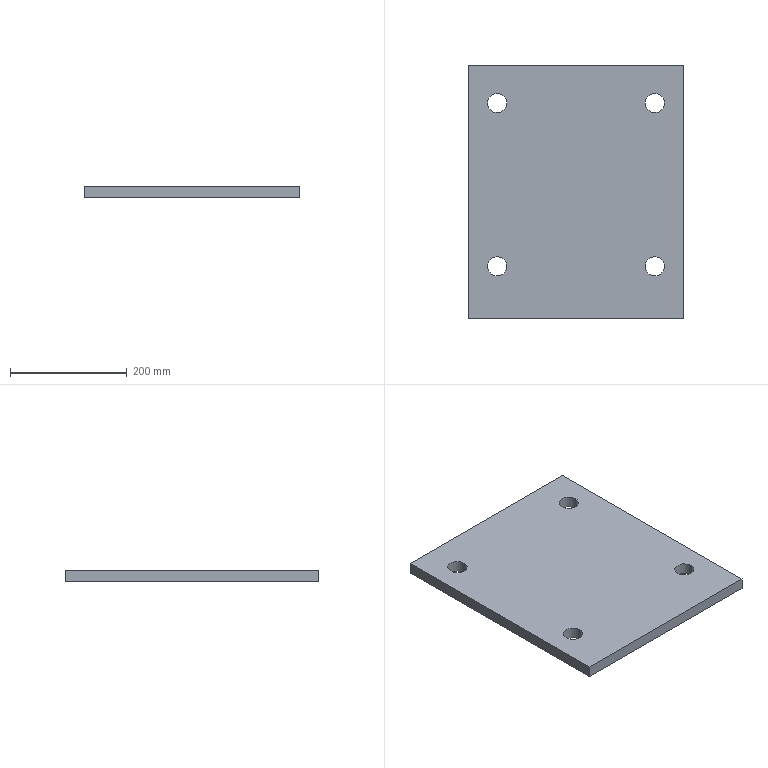Part | STEP file | Motor fixing plate | 1 solid | 14 faces | box 370 x 435 x 20 mm | volume 3150576 mm3 | cylinder 8 | plane 6 | commonest cylinder face diameters 33 x8
STEP:
#1=CARTESIAN_POINT('',(0.,0.,0.));
#2=DIRECTION('',(0.,0.,1.));
#3=DIRECTION('',(1.,0.,0.));
#4=AXIS2_PLACEMENT_3D('',#1,#2,#3);
#5=CARTESIAN_POINT('',(33.5,-345.,20.));
#6=VERTEX_POINT('',#5);
#7=CARTESIAN_POINT('',(33.5,-345.,0.));
#8=VERTEX_POINT('',#7);
#9=CARTESIAN_POINT('',(33.5,-345.,20.));
#10=DIRECTION('',(0.,0.,-1.));
#11=VECTOR('',#10,1.);
#12=LINE('',#9,#11);
#13=CARTESIAN_POINT('',(50.,-345.,20.));
#14=DIRECTION('',(0.,0.,-1.));
#15=DIRECTION('',(-1.,0.,0.));
#16=AXIS2_PLACEMENT_3D('',#13,#14,#15);
#17=CYLINDRICAL_SURFACE('',#16,16.5);
#18=CARTESIAN_POINT('',(6.283,0.));
#19=DIRECTION('',(0.,1.));
#20=VECTOR('',#19,1.);
#21=LINE('',#18,#20);
#22=(GEOMETRIC_REPRESENTATION_CONTEXT(2)PARAMETRIC_REPRESENTATION_CONTEXT()REPRESENTATION_CONTEXT('',''));
#23=DEFINITIONAL_REPRESENTATION('',(#21),#22);
#24=PCURVE('',#17,#23);
#25=CARTESIAN_POINT('',(50.,-345.,20.));
#26=DIRECTION('',(0.,0.,-1.));
#27=DIRECTION('',(-1.,0.,0.));
#28=AXIS2_PLACEMENT_3D('',#25,#26,#27);
#29=CYLINDRICAL_SURFACE('',#28,16.5);
#30=CARTESIAN_POINT('',(0.,0.));
#31=DIRECTION('',(0.,1.));
#32=VECTOR('',#31,1.);
#33=LINE('',#30,#32);
#34=(GEOMETRIC_REPRESENTATION_CONTEXT(2)PARAMETRIC_REPRESENTATION_CONTEXT()REPRESENTATION_CONTEXT('',''));
#35=DEFINITIONAL_REPRESENTATION('',(#33),#34);
#36=PCURVE('',#29,#35);
#37=SURFACE_CURVE('',#12,(#24,#36),.PCURVE_S1.);
#38=EDGE_CURVE('',#6,#8,#37,.T.);
#39=ORIENTED_EDGE('',*,*,#38,.T.);
#40=CARTESIAN_POINT('',(66.5,-345.,0.));
#41=VERTEX_POINT('',#40);
#42=CARTESIAN_POINT('',(50.,-345.,0.));
#43=DIRECTION('',(0.,0.,1.));
#44=DIRECTION('',(1.,0.,0.));
#45=AXIS2_PLACEMENT_3D('',#42,#43,#44);
#46=CIRCLE('',#45,16.5);
#47=CARTESIAN_POINT('',(9.425,20.));
#48=DIRECTION('',(-1.,0.));
#49=VECTOR('',#48,1.);
#50=LINE('',#47,#49);
#51=(GEOMETRIC_REPRESENTATION_CONTEXT(2)PARAMETRIC_REPRESENTATION_CONTEXT()REPRESENTATION_CONTEXT('',''));
#52=DEFINITIONAL_REPRESENTATION('',(#50),#51);
#53=PCURVE('',#17,#52);
#54=CARTESIAN_POINT('',(0.,0.,0.));
#55=DIRECTION('',(0.,0.,1.));
#56=DIRECTION('',(1.,0.,0.));
#57=AXIS2_PLACEMENT_3D('',#54,#55,#56);
#58=PLANE('',#57);
#59=CARTESIAN_POINT('',(50.,-345.));
#60=DIRECTION('',(1.,0.));
#61=AXIS2_PLACEMENT_2D('',#59,#60);
#62=CIRCLE('',#61,16.5);
#63=(GEOMETRIC_REPRESENTATION_CONTEXT(2)PARAMETRIC_REPRESENTATION_CONTEXT()REPRESENTATION_CONTEXT('',''));
#64=DEFINITIONAL_REPRESENTATION('',(#62),#63);
#65=PCURVE('',#58,#64);
#66=SURFACE_CURVE('',#46,(#53,#65),.PCURVE_S1.);
#67=EDGE_CURVE('',#8,#41,#66,.T.);
#68=ORIENTED_EDGE('',*,*,#67,.T.);
#69=CARTESIAN_POINT('',(66.5,-345.,20.));
#70=VERTEX_POINT('',#69);
#71=CARTESIAN_POINT('',(66.5,-345.,20.));
#72=DIRECTION('',(0.,0.,-1.));
#73=VECTOR('',#72,1.);
#74=LINE('',#71,#73);
#75=CARTESIAN_POINT('',(3.142,0.));
#76=DIRECTION('',(0.,1.));
#77=VECTOR('',#76,1.);
#78=LINE('',#75,#77);
#79=(GEOMETRIC_REPRESENTATION_CONTEXT(2)PARAMETRIC_REPRESENTATION_CONTEXT()REPRESENTATION_CONTEXT('',''));
#80=DEFINITIONAL_REPRESENTATION('',(#78),#79);
#81=PCURVE('',#17,#80);
#82=CARTESIAN_POINT('',(3.142,0.));
#83=DIRECTION('',(0.,1.));
#84=VECTOR('',#83,1.);
#85=LINE('',#82,#84);
#86=(GEOMETRIC_REPRESENTATION_CONTEXT(2)PARAMETRIC_REPRESENTATION_CONTEXT()REPRESENTATION_CONTEXT('',''));
#87=DEFINITIONAL_REPRESENTATION('',(#85),#86);
#88=PCURVE('',#29,#87);
#89=SURFACE_CURVE('',#74,(#81,#88),.PCURVE_S1.);
#90=EDGE_CURVE('',#70,#41,#89,.T.);
#91=ORIENTED_EDGE('',*,*,#90,.F.);
#92=CARTESIAN_POINT('',(50.,-345.,20.));
#93=DIRECTION('',(0.,0.,1.));
#94=DIRECTION('',(1.,0.,0.));
#95=AXIS2_PLACEMENT_3D('',#92,#93,#94);
#96=CIRCLE('',#95,16.5);
#97=CARTESIAN_POINT('',(9.425,0.));
#98=DIRECTION('',(-1.,0.));
#99=VECTOR('',#98,1.);
#100=LINE('',#97,#99);
#101=(GEOMETRIC_REPRESENTATION_CONTEXT(2)PARAMETRIC_REPRESENTATION_CONTEXT()REPRESENTATION_CONTEXT('',''));
#102=DEFINITIONAL_REPRESENTATION('',(#100),#101);
#103=PCURVE('',#17,#102);
#104=CARTESIAN_POINT('',(0.,0.,20.));
#105=DIRECTION('',(0.,0.,1.));
#106=DIRECTION('',(1.,0.,0.));
#107=AXIS2_PLACEMENT_3D('',#104,#105,#106);
#108=PLANE('',#107);
#109=CARTESIAN_POINT('',(50.,-345.));
#110=DIRECTION('',(1.,0.));
#111=AXIS2_PLACEMENT_2D('',#109,#110);
#112=CIRCLE('',#111,16.5);
#113=(GEOMETRIC_REPRESENTATION_CONTEXT(2)PARAMETRIC_REPRESENTATION_CONTEXT()REPRESENTATION_CONTEXT('',''));
#114=DEFINITIONAL_REPRESENTATION('',(#112),#113);
#115=PCURVE('',#108,#114);
#116=SURFACE_CURVE('',#96,(#103,#115),.PCURVE_S1.);
#117=EDGE_CURVE('',#6,#70,#116,.T.);
#118=ORIENTED_EDGE('',*,*,#117,.F.);
#119=EDGE_LOOP('',(#39,#68,#91,#118));
#120=FACE_BOUND('',#119,.F.);
#121=ADVANCED_FACE('',(#120),#17,.F.);
#122=CARTESIAN_POINT('',(303.5,-345.,20.));
#123=VERTEX_POINT('',#122);
#124=CARTESIAN_POINT('',(303.5,-345.,0.));
#125=VERTEX_POINT('',#124);
#126=CARTESIAN_POINT('',(303.5,-345.,20.));
#127=DIRECTION('',(0.,0.,-1.));
#128=VECTOR('',#127,1.);
#129=LINE('',#126,#128);
#130=CARTESIAN_POINT('',(320.,-345.,20.));
#131=DIRECTION('',(0.,0.,-1.));
#132=DIRECTION('',(-1.,0.,0.));
#133=AXIS2_PLACEMENT_3D('',#130,#131,#132);
#134=CYLINDRICAL_SURFACE('',#133,16.5);
#135=CARTESIAN_POINT('',(6.283,0.));
#136=DIRECTION('',(0.,1.));
#137=VECTOR('',#136,1.);
#138=LINE('',#135,#137);
#139=(GEOMETRIC_REPRESENTATION_CONTEXT(2)PARAMETRIC_REPRESENTATION_CONTEXT()REPRESENTATION_CONTEXT('',''));
#140=DEFINITIONAL_REPRESENTATION('',(#138),#139);
#141=PCURVE('',#134,#140);
#142=CARTESIAN_POINT('',(320.,-345.,20.));
#143=DIRECTION('',(0.,0.,-1.));
#144=DIRECTION('',(-1.,0.,0.));
#145=AXIS2_PLACEMENT_3D('',#142,#143,#144);
#146=CYLINDRICAL_SURFACE('',#145,16.5);
#147=CARTESIAN_POINT('',(0.,0.));
#148=DIRECTION('',(0.,1.));
#149=VECTOR('',#148,1.);
#150=LINE('',#147,#149);
#151=(GEOMETRIC_REPRESENTATION_CONTEXT(2)PARAMETRIC_REPRESENTATION_CONTEXT()REPRESENTATION_CONTEXT('',''));
#152=DEFINITIONAL_REPRESENTATION('',(#150),#151);
#153=PCURVE('',#146,#152);
#154=SURFACE_CURVE('',#129,(#141,#153),.PCURVE_S1.);
#155=EDGE_CURVE('',#123,#125,#154,.T.);
#156=ORIENTED_EDGE('',*,*,#155,.T.);
#157=CARTESIAN_POINT('',(336.5,-345.,0.));
#158=VERTEX_POINT('',#157);
#159=CARTESIAN_POINT('',(320.,-345.,0.));
#160=DIRECTION('',(0.,0.,1.));
#161=DIRECTION('',(1.,0.,0.));
#162=AXIS2_PLACEMENT_3D('',#159,#160,#161);
#163=CIRCLE('',#162,16.5);
#164=CARTESIAN_POINT('',(9.425,20.));
#165=DIRECTION('',(-1.,0.));
#166=VECTOR('',#165,1.);
#167=LINE('',#164,#166);
#168=(GEOMETRIC_REPRESENTATION_CONTEXT(2)PARAMETRIC_REPRESENTATION_CONTEXT()REPRESENTATION_CONTEXT('',''));
#169=DEFINITIONAL_REPRESENTATION('',(#167),#168);
#170=PCURVE('',#134,#169);
#171=CARTESIAN_POINT('',(320.,-345.));
#172=DIRECTION('',(1.,0.));
#173=AXIS2_PLACEMENT_2D('',#171,#172);
#174=CIRCLE('',#173,16.5);
#175=(GEOMETRIC_REPRESENTATION_CONTEXT(2)PARAMETRIC_REPRESENTATION_CONTEXT()REPRESENTATION_CONTEXT('',''));
#176=DEFINITIONAL_REPRESENTATION('',(#174),#175);
#177=PCURVE('',#58,#176);
#178=SURFACE_CURVE('',#163,(#170,#177),.PCURVE_S1.);
#179=EDGE_CURVE('',#125,#158,#178,.T.);
#180=ORIENTED_EDGE('',*,*,#179,.T.);
#181=CARTESIAN_POINT('',(336.5,-345.,20.));
#182=VERTEX_POINT('',#181);
#183=CARTESIAN_POINT('',(336.5,-345.,20.));
#184=DIRECTION('',(0.,0.,-1.));
#185=VECTOR('',#184,1.);
#186=LINE('',#183,#185);
#187=CARTESIAN_POINT('',(3.142,0.));
#188=DIRECTION('',(0.,1.));
#189=VECTOR('',#188,1.);
#190=LINE('',#187,#189);
#191=(GEOMETRIC_REPRESENTATION_CONTEXT(2)PARAMETRIC_REPRESENTATION_CONTEXT()REPRESENTATION_CONTEXT('',''));
#192=DEFINITIONAL_REPRESENTATION('',(#190),#191);
#193=PCURVE('',#134,#192);
#194=CARTESIAN_POINT('',(3.142,0.));
#195=DIRECTION('',(0.,1.));
#196=VECTOR('',#195,1.);
#197=LINE('',#194,#196);
#198=(GEOMETRIC_REPRESENTATION_CONTEXT(2)PARAMETRIC_REPRESENTATION_CONTEXT()REPRESENTATION_CONTEXT('',''));
#199=DEFINITIONAL_REPRESENTATION('',(#197),#198);
#200=PCURVE('',#146,#199);
#201=SURFACE_CURVE('',#186,(#193,#200),.PCURVE_S1.);
#202=EDGE_CURVE('',#182,#158,#201,.T.);
#203=ORIENTED_EDGE('',*,*,#202,.F.);
#204=CARTESIAN_POINT('',(320.,-345.,20.));
#205=DIRECTION('',(0.,0.,1.));
#206=DIRECTION('',(1.,0.,0.));
#207=AXIS2_PLACEMENT_3D('',#204,#205,#206);
#208=CIRCLE('',#207,16.5);
#209=CARTESIAN_POINT('',(9.425,0.));
#210=DIRECTION('',(-1.,0.));
#211=VECTOR('',#210,1.);
#212=LINE('',#209,#211);
#213=(GEOMETRIC_REPRESENTATION_CONTEXT(2)PARAMETRIC_REPRESENTATION_CONTEXT()REPRESENTATION_CONTEXT('',''));
#214=DEFINITIONAL_REPRESENTATION('',(#212),#213);
#215=PCURVE('',#134,#214);
#216=CARTESIAN_POINT('',(320.,-345.));
#217=DIRECTION('',(1.,0.));
#218=AXIS2_PLACEMENT_2D('',#216,#217);
#219=CIRCLE('',#218,16.5);
#220=(GEOMETRIC_REPRESENTATION_CONTEXT(2)PARAMETRIC_REPRESENTATION_CONTEXT()REPRESENTATION_CONTEXT('',''));
#221=DEFINITIONAL_REPRESENTATION('',(#219),#220);
#222=PCURVE('',#108,#221);
#223=SURFACE_CURVE('',#208,(#215,#222),.PCURVE_S1.);
#224=EDGE_CURVE('',#123,#182,#223,.T.);
#225=ORIENTED_EDGE('',*,*,#224,.F.);
#226=EDGE_LOOP('',(#156,#180,#203,#225));
#227=FACE_BOUND('',#226,.F.);
#228=ADVANCED_FACE('',(#227),#134,.F.);
#229=CARTESIAN_POINT('',(303.5,-65.,20.));
#230=VERTEX_POINT('',#229);
#231=CARTESIAN_POINT('',(303.5,-65.,0.));
#232=VERTEX_POINT('',#231);
#233=CARTESIAN_POINT('',(303.5,-65.,20.));
#234=DIRECTION('',(0.,0.,-1.));
#235=VECTOR('',#234,1.);
#236=LINE('',#233,#235);
#237=CARTESIAN_POINT('',(320.,-65.,20.));
#238=DIRECTION('',(0.,0.,-1.));
#239=DIRECTION('',(-1.,0.,0.));
#240=AXIS2_PLACEMENT_3D('',#237,#238,#239);
#241=CYLINDRICAL_SURFACE('',#240,16.5);
#242=CARTESIAN_POINT('',(6.283,0.));
#243=DIRECTION('',(0.,1.));
#244=VECTOR('',#243,1.);
#245=LINE('',#242,#244);
#246=(GEOMETRIC_REPRESENTATION_CONTEXT(2)PARAMETRIC_REPRESENTATION_CONTEXT()REPRESENTATION_CONTEXT('',''));
#247=DEFINITIONAL_REPRESENTATION('',(#245),#246);
#248=PCURVE('',#241,#247);
#249=CARTESIAN_POINT('',(320.,-65.,20.));
#250=DIRECTION('',(0.,0.,-1.));
#251=DIRECTION('',(-1.,0.,0.));
#252=AXIS2_PLACEMENT_3D('',#249,#250,#251);
#253=CYLINDRICAL_SURFACE('',#252,16.5);
#254=CARTESIAN_POINT('',(0.,0.));
#255=DIRECTION('',(0.,1.));
#256=VECTOR('',#255,1.);
#257=LINE('',#254,#256);
#258=(GEOMETRIC_REPRESENTATION_CONTEXT(2)PARAMETRIC_REPRESENTATION_CONTEXT()REPRESENTATION_CONTEXT('',''));
#259=DEFINITIONAL_REPRESENTATION('',(#257),#258);
#260=PCURVE('',#253,#259);
#261=SURFACE_CURVE('',#236,(#248,#260),.PCURVE_S1.);
#262=EDGE_CURVE('',#230,#232,#261,.T.);
#263=ORIENTED_EDGE('',*,*,#262,.T.);
#264=CARTESIAN_POINT('',(336.5,-65.,0.));
#265=VERTEX_POINT('',#264);
#266=CARTESIAN_POINT('',(320.,-65.,0.));
#267=DIRECTION('',(0.,0.,1.));
#268=DIRECTION('',(1.,0.,0.));
#269=AXIS2_PLACEMENT_3D('',#266,#267,#268);
#270=CIRCLE('',#269,16.5);
#271=CARTESIAN_POINT('',(9.425,20.));
#272=DIRECTION('',(-1.,0.));
#273=VECTOR('',#272,1.);
#274=LINE('',#271,#273);
#275=(GEOMETRIC_REPRESENTATION_CONTEXT(2)PARAMETRIC_REPRESENTATION_CONTEXT()REPRESENTATION_CONTEXT('',''));
#276=DEFINITIONAL_REPRESENTATION('',(#274),#275);
#277=PCURVE('',#241,#276);
#278=CARTESIAN_POINT('',(320.,-65.));
#279=DIRECTION('',(1.,0.));
#280=AXIS2_PLACEMENT_2D('',#278,#279);
#281=CIRCLE('',#280,16.5);
#282=(GEOMETRIC_REPRESENTATION_CONTEXT(2)PARAMETRIC_REPRESENTATION_CONTEXT()REPRESENTATION_CONTEXT('',''));
#283=DEFINITIONAL_REPRESENTATION('',(#281),#282);
#284=PCURVE('',#58,#283);
#285=SURFACE_CURVE('',#270,(#277,#284),.PCURVE_S1.);
#286=EDGE_CURVE('',#232,#265,#285,.T.);
#287=ORIENTED_EDGE('',*,*,#286,.T.);
#288=CARTESIAN_POINT('',(336.5,-65.,20.));
#289=VERTEX_POINT('',#288);
#290=CARTESIAN_POINT('',(336.5,-65.,20.));
#291=DIRECTION('',(0.,0.,-1.));
#292=VECTOR('',#291,1.);
#293=LINE('',#290,#292);
#294=CARTESIAN_POINT('',(3.142,0.));
#295=DIRECTION('',(0.,1.));
#296=VECTOR('',#295,1.);
#297=LINE('',#294,#296);
#298=(GEOMETRIC_REPRESENTATION_CONTEXT(2)PARAMETRIC_REPRESENTATION_CONTEXT()REPRESENTATION_CONTEXT('',''));
#299=DEFINITIONAL_REPRESENTATION('',(#297),#298);
#300=PCURVE('',#241,#299);
#301=CARTESIAN_POINT('',(3.142,0.));
#302=DIRECTION('',(0.,1.));
#303=VECTOR('',#302,1.);
#304=LINE('',#301,#303);
#305=(GEOMETRIC_REPRESENTATION_CONTEXT(2)PARAMETRIC_REPRESENTATION_CONTEXT()REPRESENTATION_CONTEXT('',''));
#306=DEFINITIONAL_REPRESENTATION('',(#304),#305);
#307=PCURVE('',#253,#306);
#308=SURFACE_CURVE('',#293,(#300,#307),.PCURVE_S1.);
#309=EDGE_CURVE('',#289,#265,#308,.T.);
#310=ORIENTED_EDGE('',*,*,#309,.F.);
#311=CARTESIAN_POINT('',(320.,-65.,20.));
#312=DIRECTION('',(0.,0.,1.));
#313=DIRECTION('',(1.,0.,0.));
#314=AXIS2_PLACEMENT_3D('',#311,#312,#313);
#315=CIRCLE('',#314,16.5);
#316=CARTESIAN_POINT('',(9.425,0.));
#317=DIRECTION('',(-1.,0.));
#318=VECTOR('',#317,1.);
#319=LINE('',#316,#318);
#320=(GEOMETRIC_REPRESENTATION_CONTEXT(2)PARAMETRIC_REPRESENTATION_CONTEXT()REPRESENTATION_CONTEXT('',''));
#321=DEFINITIONAL_REPRESENTATION('',(#319),#320);
#322=PCURVE('',#241,#321);
#323=CARTESIAN_POINT('',(320.,-65.));
#324=DIRECTION('',(1.,0.));
#325=AXIS2_PLACEMENT_2D('',#323,#324);
#326=CIRCLE('',#325,16.5);
#327=(GEOMETRIC_REPRESENTATION_CONTEXT(2)PARAMETRIC_REPRESENTATION_CONTEXT()REPRESENTATION_CONTEXT('',''));
#328=DEFINITIONAL_REPRESENTATION('',(#326),#327);
#329=PCURVE('',#108,#328);
#330=SURFACE_CURVE('',#315,(#322,#329),.PCURVE_S1.);
#331=EDGE_CURVE('',#230,#289,#330,.T.);
#332=ORIENTED_EDGE('',*,*,#331,.F.);
#333=EDGE_LOOP('',(#263,#287,#310,#332));
#334=FACE_BOUND('',#333,.F.);
#335=ADVANCED_FACE('',(#334),#241,.F.);
#336=CARTESIAN_POINT('',(33.5,-65.,20.));
#337=VERTEX_POINT('',#336);
#338=CARTESIAN_POINT('',(33.5,-65.,0.));
#339=VERTEX_POINT('',#338);
#340=CARTESIAN_POINT('',(33.5,-65.,20.));
#341=DIRECTION('',(0.,0.,-1.));
#342=VECTOR('',#341,1.);
#343=LINE('',#340,#342);
#344=CARTESIAN_POINT('',(50.,-65.,20.));
#345=DIRECTION('',(0.,0.,-1.));
#346=DIRECTION('',(-1.,0.,0.));
#347=AXIS2_PLACEMENT_3D('',#344,#345,#346);
#348=CYLINDRICAL_SURFACE('',#347,16.5);
#349=CARTESIAN_POINT('',(6.283,0.));
#350=DIRECTION('',(0.,1.));
#351=VECTOR('',#350,1.);
#352=LINE('',#349,#351);
#353=(GEOMETRIC_REPRESENTATION_CONTEXT(2)PARAMETRIC_REPRESENTATION_CONTEXT()REPRESENTATION_CONTEXT('',''));
#354=DEFINITIONAL_REPRESENTATION('',(#352),#353);
#355=PCURVE('',#348,#354);
#356=CARTESIAN_POINT('',(50.,-65.,20.));
#357=DIRECTION('',(0.,0.,-1.));
#358=DIRECTION('',(-1.,0.,0.));
#359=AXIS2_PLACEMENT_3D('',#356,#357,#358);
#360=CYLINDRICAL_SURFACE('',#359,16.5);
#361=CARTESIAN_POINT('',(0.,0.));
#362=DIRECTION('',(0.,1.));
#363=VECTOR('',#362,1.);
#364=LINE('',#361,#363);
#365=(GEOMETRIC_REPRESENTATION_CONTEXT(2)PARAMETRIC_REPRESENTATION_CONTEXT()REPRESENTATION_CONTEXT('',''));
#366=DEFINITIONAL_REPRESENTATION('',(#364),#365);
#367=PCURVE('',#360,#366);
#368=SURFACE_CURVE('',#343,(#355,#367),.PCURVE_S1.);
#369=EDGE_CURVE('',#337,#339,#368,.T.);
#370=ORIENTED_EDGE('',*,*,#369,.T.);
#371=CARTESIAN_POINT('',(66.5,-65.,0.));
#372=VERTEX_POINT('',#371);
#373=CARTESIAN_POINT('',(50.,-65.,0.));
#374=DIRECTION('',(0.,0.,1.));
#375=DIRECTION('',(1.,0.,0.));
#376=AXIS2_PLACEMENT_3D('',#373,#374,#375);
#377=CIRCLE('',#376,16.5);
#378=CARTESIAN_POINT('',(9.425,20.));
#379=DIRECTION('',(-1.,0.));
#380=VECTOR('',#379,1.);
#381=LINE('',#378,#380);
#382=(GEOMETRIC_REPRESENTATION_CONTEXT(2)PARAMETRIC_REPRESENTATION_CONTEXT()REPRESENTATION_CONTEXT('',''));
#383=DEFINITIONAL_REPRESENTATION('',(#381),#382);
#384=PCURVE('',#348,#383);
#385=CARTESIAN_POINT('',(50.,-65.));
#386=DIRECTION('',(1.,0.));
#387=AXIS2_PLACEMENT_2D('',#385,#386);
#388=CIRCLE('',#387,16.5);
#389=(GEOMETRIC_REPRESENTATION_CONTEXT(2)PARAMETRIC_REPRESENTATION_CONTEXT()REPRESENTATION_CONTEXT('',''));
#390=DEFINITIONAL_REPRESENTATION('',(#388),#389);
#391=PCURVE('',#58,#390);
#392=SURFACE_CURVE('',#377,(#384,#391),.PCURVE_S1.);
#393=EDGE_CURVE('',#339,#372,#392,.T.);
#394=ORIENTED_EDGE('',*,*,#393,.T.);
#395=CARTESIAN_POINT('',(66.5,-65.,20.));
#396=VERTEX_POINT('',#395);
#397=CARTESIAN_POINT('',(66.5,-65.,20.));
#398=DIRECTION('',(0.,0.,-1.));
#399=VECTOR('',#398,1.);
#400=LINE('',#397,#399);
#401=CARTESIAN_POINT('',(3.142,0.));
#402=DIRECTION('',(0.,1.));
#403=VECTOR('',#402,1.);
#404=LINE('',#401,#403);
#405=(GEOMETRIC_REPRESENTATION_CONTEXT(2)PARAMETRIC_REPRESENTATION_CONTEXT()REPRESENTATION_CONTEXT('',''));
#406=DEFINITIONAL_REPRESENTATION('',(#404),#405);
#407=PCURVE('',#348,#406);
#408=CARTESIAN_POINT('',(3.142,0.));
#409=DIRECTION('',(0.,1.));
#410=VECTOR('',#409,1.);
#411=LINE('',#408,#410);
#412=(GEOMETRIC_REPRESENTATION_CONTEXT(2)PARAMETRIC_REPRESENTATION_CONTEXT()REPRESENTATION_CONTEXT('',''));
#413=DEFINITIONAL_REPRESENTATION('',(#411),#412);
#414=PCURVE('',#360,#413);
#415=SURFACE_CURVE('',#400,(#407,#414),.PCURVE_S1.);
#416=EDGE_CURVE('',#396,#372,#415,.T.);
#417=ORIENTED_EDGE('',*,*,#416,.F.);
#418=CARTESIAN_POINT('',(50.,-65.,20.));
#419=DIRECTION('',(0.,0.,1.));
#420=DIRECTION('',(1.,0.,0.));
#421=AXIS2_PLACEMENT_3D('',#418,#419,#420);
#422=CIRCLE('',#421,16.5);
#423=CARTESIAN_POINT('',(9.425,0.));
#424=DIRECTION('',(-1.,0.));
#425=VECTOR('',#424,1.);
#426=LINE('',#423,#425);
#427=(GEOMETRIC_REPRESENTATION_CONTEXT(2)PARAMETRIC_REPRESENTATION_CONTEXT()REPRESENTATION_CONTEXT('',''));
#428=DEFINITIONAL_REPRESENTATION('',(#426),#427);
#429=PCURVE('',#348,#428);
#430=CARTESIAN_POINT('',(50.,-65.));
#431=DIRECTION('',(1.,0.));
#432=AXIS2_PLACEMENT_2D('',#430,#431);
#433=CIRCLE('',#432,16.5);
#434=(GEOMETRIC_REPRESENTATION_CONTEXT(2)PARAMETRIC_REPRESENTATION_CONTEXT()REPRESENTATION_CONTEXT('',''));
#435=DEFINITIONAL_REPRESENTATION('',(#433),#434);
#436=PCURVE('',#108,#435);
#437=SURFACE_CURVE('',#422,(#429,#436),.PCURVE_S1.);
#438=EDGE_CURVE('',#337,#396,#437,.T.);
#439=ORIENTED_EDGE('',*,*,#438,.F.);
#440=EDGE_LOOP('',(#370,#394,#417,#439));
#441=FACE_BOUND('',#440,.F.);
#442=ADVANCED_FACE('',(#441),#348,.F.);
#443=ORIENTED_EDGE('',*,*,#224,.F.);
#444=CARTESIAN_POINT('',(320.,-345.,20.));
#445=DIRECTION('',(0.,0.,1.));
#446=DIRECTION('',(1.,0.,0.));
#447=AXIS2_PLACEMENT_3D('',#444,#445,#446);
#448=CIRCLE('',#447,16.5);
#449=CARTESIAN_POINT('',(320.,-345.));
#450=DIRECTION('',(1.,0.));
#451=AXIS2_PLACEMENT_2D('',#449,#450);
#452=CIRCLE('',#451,16.5);
#453=(GEOMETRIC_REPRESENTATION_CONTEXT(2)PARAMETRIC_REPRESENTATION_CONTEXT()REPRESENTATION_CONTEXT('',''));
#454=DEFINITIONAL_REPRESENTATION('',(#452),#453);
#455=PCURVE('',#108,#454);
#456=CARTESIAN_POINT('',(3.142,0.));
#457=DIRECTION('',(-1.,0.));
#458=VECTOR('',#457,1.);
#459=LINE('',#456,#458);
#460=(GEOMETRIC_REPRESENTATION_CONTEXT(2)PARAMETRIC_REPRESENTATION_CONTEXT()REPRESENTATION_CONTEXT('',''));
#461=DEFINITIONAL_REPRESENTATION('',(#459),#460);
#462=PCURVE('',#146,#461);
#463=SURFACE_CURVE('',#448,(#455,#462),.PCURVE_S1.);
#464=EDGE_CURVE('',#182,#123,#463,.T.);
#465=ORIENTED_EDGE('',*,*,#464,.F.);
#466=EDGE_LOOP('',(#443,#465));
#467=FACE_BOUND('',#466,.T.);
#468=ORIENTED_EDGE('',*,*,#438,.F.);
#469=CARTESIAN_POINT('',(50.,-65.,20.));
#470=DIRECTION('',(0.,0.,1.));
#471=DIRECTION('',(1.,0.,0.));
#472=AXIS2_PLACEMENT_3D('',#469,#470,#471);
#473=CIRCLE('',#472,16.5);
#474=CARTESIAN_POINT('',(50.,-65.));
#475=DIRECTION('',(1.,0.));
#476=AXIS2_PLACEMENT_2D('',#474,#475);
#477=CIRCLE('',#476,16.5);
#478=(GEOMETRIC_REPRESENTATION_CONTEXT(2)PARAMETRIC_REPRESENTATION_CONTEXT()REPRESENTATION_CONTEXT('',''));
#479=DEFINITIONAL_REPRESENTATION('',(#477),#478);
#480=PCURVE('',#108,#479);
#481=CARTESIAN_POINT('',(3.142,0.));
#482=DIRECTION('',(-1.,0.));
#483=VECTOR('',#482,1.);
#484=LINE('',#481,#483);
#485=(GEOMETRIC_REPRESENTATION_CONTEXT(2)PARAMETRIC_REPRESENTATION_CONTEXT()REPRESENTATION_CONTEXT('',''));
#486=DEFINITIONAL_REPRESENTATION('',(#484),#485);
#487=PCURVE('',#360,#486);
#488=SURFACE_CURVE('',#473,(#480,#487),.PCURVE_S1.);
#489=EDGE_CURVE('',#396,#337,#488,.T.);
#490=ORIENTED_EDGE('',*,*,#489,.F.);
#491=EDGE_LOOP('',(#468,#490));
#492=FACE_BOUND('',#491,.T.);
#493=CARTESIAN_POINT('',(0.,0.,20.));
#494=VERTEX_POINT('',#493);
#495=CARTESIAN_POINT('',(0.,-435.,20.));
#496=VERTEX_POINT('',#495);
#497=CARTESIAN_POINT('',(0.,0.,20.));
#498=DIRECTION('',(0.,-1.,0.));
#499=VECTOR('',#498,1.);
#500=LINE('',#497,#499);
#501=CARTESIAN_POINT('',(0.,0.));
#502=DIRECTION('',(0.,-1.));
#503=VECTOR('',#502,1.);
#504=LINE('',#501,#503);
#505=(GEOMETRIC_REPRESENTATION_CONTEXT(2)PARAMETRIC_REPRESENTATION_CONTEXT()REPRESENTATION_CONTEXT('',''));
#506=DEFINITIONAL_REPRESENTATION('',(#504),#505);
#507=PCURVE('',#108,#506);
#508=CARTESIAN_POINT('',(0.,0.,20.));
#509=DIRECTION('',(1.,0.,0.));
#510=DIRECTION('',(0.,1.,0.));
#511=AXIS2_PLACEMENT_3D('',#508,#509,#510);
#512=PLANE('',#511);
#513=CARTESIAN_POINT('',(0.,0.));
#514=DIRECTION('',(-1.,0.));
#515=VECTOR('',#514,1.);
#516=LINE('',#513,#515);
#517=(GEOMETRIC_REPRESENTATION_CONTEXT(2)PARAMETRIC_REPRESENTATION_CONTEXT()REPRESENTATION_CONTEXT('',''));
#518=DEFINITIONAL_REPRESENTATION('',(#516),#517);
#519=PCURVE('',#512,#518);
#520=SURFACE_CURVE('',#500,(#507,#519),.PCURVE_S1.);
#521=EDGE_CURVE('',#494,#496,#520,.T.);
#522=ORIENTED_EDGE('',*,*,#521,.T.);
#523=CARTESIAN_POINT('',(370.,-435.,20.));
#524=VERTEX_POINT('',#523);
#525=CARTESIAN_POINT('',(0.,-435.,20.));
#526=DIRECTION('',(1.,0.,0.));
#527=VECTOR('',#526,1.);
#528=LINE('',#525,#527);
#529=CARTESIAN_POINT('',(0.,-435.));
#530=DIRECTION('',(1.,0.));
#531=VECTOR('',#530,1.);
#532=LINE('',#529,#531);
#533=(GEOMETRIC_REPRESENTATION_CONTEXT(2)PARAMETRIC_REPRESENTATION_CONTEXT()REPRESENTATION_CONTEXT('',''));
#534=DEFINITIONAL_REPRESENTATION('',(#532),#533);
#535=PCURVE('',#108,#534);
#536=CARTESIAN_POINT('',(0.,-435.,20.));
#537=DIRECTION('',(0.,1.,0.));
#538=DIRECTION('',(0.,0.,1.));
#539=AXIS2_PLACEMENT_3D('',#536,#537,#538);
#540=PLANE('',#539);
#541=CARTESIAN_POINT('',(0.,0.));
#542=DIRECTION('',(0.,1.));
#543=VECTOR('',#542,1.);
#544=LINE('',#541,#543);
#545=(GEOMETRIC_REPRESENTATION_CONTEXT(2)PARAMETRIC_REPRESENTATION_CONTEXT()REPRESENTATION_CONTEXT('',''));
#546=DEFINITIONAL_REPRESENTATION('',(#544),#545);
#547=PCURVE('',#540,#546);
#548=SURFACE_CURVE('',#528,(#535,#547),.PCURVE_S1.);
#549=EDGE_CURVE('',#496,#524,#548,.T.);
#550=ORIENTED_EDGE('',*,*,#549,.T.);
#551=CARTESIAN_POINT('',(370.,0.,20.));
#552=VERTEX_POINT('',#551);
#553=CARTESIAN_POINT('',(370.,0.,20.));
#554=DIRECTION('',(0.,1.,0.));
#555=VECTOR('',#554,1.);
#556=LINE('',#553,#555);
#557=CARTESIAN_POINT('',(370.,0.));
#558=DIRECTION('',(0.,1.));
#559=VECTOR('',#558,1.);
#560=LINE('',#557,#559);
#561=(GEOMETRIC_REPRESENTATION_CONTEXT(2)PARAMETRIC_REPRESENTATION_CONTEXT()REPRESENTATION_CONTEXT('',''));
#562=DEFINITIONAL_REPRESENTATION('',(#560),#561);
#563=PCURVE('',#108,#562);
#564=CARTESIAN_POINT('',(370.,0.,20.));
#565=DIRECTION('',(-1.,0.,0.));
#566=DIRECTION('',(0.,-1.,0.));
#567=AXIS2_PLACEMENT_3D('',#564,#565,#566);
#568=PLANE('',#567);
#569=CARTESIAN_POINT('',(0.,0.));
#570=DIRECTION('',(-1.,0.));
#571=VECTOR('',#570,1.);
#572=LINE('',#569,#571);
#573=(GEOMETRIC_REPRESENTATION_CONTEXT(2)PARAMETRIC_REPRESENTATION_CONTEXT()REPRESENTATION_CONTEXT('',''));
#574=DEFINITIONAL_REPRESENTATION('',(#572),#573);
#575=PCURVE('',#568,#574);
#576=SURFACE_CURVE('',#556,(#563,#575),.PCURVE_S1.);
#577=EDGE_CURVE('',#524,#552,#576,.T.);
#578=ORIENTED_EDGE('',*,*,#577,.T.);
#579=CARTESIAN_POINT('',(0.,0.,20.));
#580=DIRECTION('',(-1.,0.,0.));
#581=VECTOR('',#580,1.);
#582=LINE('',#579,#581);
#583=CARTESIAN_POINT('',(0.,0.));
#584=DIRECTION('',(-1.,0.));
#585=VECTOR('',#584,1.);
#586=LINE('',#583,#585);
#587=(GEOMETRIC_REPRESENTATION_CONTEXT(2)PARAMETRIC_REPRESENTATION_CONTEXT()REPRESENTATION_CONTEXT('',''));
#588=DEFINITIONAL_REPRESENTATION('',(#586),#587);
#589=PCURVE('',#108,#588);
#590=CARTESIAN_POINT('',(0.,0.,20.));
#591=DIRECTION('',(0.,-1.,0.));
#592=DIRECTION('',(0.,0.,-1.));
#593=AXIS2_PLACEMENT_3D('',#590,#591,#592);
#594=PLANE('',#593);
#595=CARTESIAN_POINT('',(0.,0.));
#596=DIRECTION('',(0.,-1.));
#597=VECTOR('',#596,1.);
#598=LINE('',#595,#597);
#599=(GEOMETRIC_REPRESENTATION_CONTEXT(2)PARAMETRIC_REPRESENTATION_CONTEXT()REPRESENTATION_CONTEXT('',''));
#600=DEFINITIONAL_REPRESENTATION('',(#598),#599);
#601=PCURVE('',#594,#600);
#602=SURFACE_CURVE('',#582,(#589,#601),.PCURVE_S1.);
#603=EDGE_CURVE('',#552,#494,#602,.T.);
#604=ORIENTED_EDGE('',*,*,#603,.T.);
#605=EDGE_LOOP('',(#522,#550,#578,#604));
#606=FACE_BOUND('',#605,.T.);
#607=ORIENTED_EDGE('',*,*,#331,.F.);
#608=CARTESIAN_POINT('',(320.,-65.,20.));
#609=DIRECTION('',(0.,0.,1.));
#610=DIRECTION('',(1.,0.,0.));
#611=AXIS2_PLACEMENT_3D('',#608,#609,#610);
#612=CIRCLE('',#611,16.5);
#613=CARTESIAN_POINT('',(320.,-65.));
#614=DIRECTION('',(1.,0.));
#615=AXIS2_PLACEMENT_2D('',#613,#614);
#616=CIRCLE('',#615,16.5);
#617=(GEOMETRIC_REPRESENTATION_CONTEXT(2)PARAMETRIC_REPRESENTATION_CONTEXT()REPRESENTATION_CONTEXT('',''));
#618=DEFINITIONAL_REPRESENTATION('',(#616),#617);
#619=PCURVE('',#108,#618);
#620=CARTESIAN_POINT('',(3.142,0.));
#621=DIRECTION('',(-1.,0.));
#622=VECTOR('',#621,1.);
#623=LINE('',#620,#622);
#624=(GEOMETRIC_REPRESENTATION_CONTEXT(2)PARAMETRIC_REPRESENTATION_CONTEXT()REPRESENTATION_CONTEXT('',''));
#625=DEFINITIONAL_REPRESENTATION('',(#623),#624);
#626=PCURVE('',#253,#625);
#627=SURFACE_CURVE('',#612,(#619,#626),.PCURVE_S1.);
#628=EDGE_CURVE('',#289,#230,#627,.T.);
#629=ORIENTED_EDGE('',*,*,#628,.F.);
#630=EDGE_LOOP('',(#607,#629));
#631=FACE_BOUND('',#630,.T.);
#632=ORIENTED_EDGE('',*,*,#117,.F.);
#633=CARTESIAN_POINT('',(50.,-345.,20.));
#634=DIRECTION('',(0.,0.,1.));
#635=DIRECTION('',(1.,0.,0.));
#636=AXIS2_PLACEMENT_3D('',#633,#634,#635);
#637=CIRCLE('',#636,16.5);
#638=CARTESIAN_POINT('',(50.,-345.));
#639=DIRECTION('',(1.,0.));
#640=AXIS2_PLACEMENT_2D('',#638,#639);
#641=CIRCLE('',#640,16.5);
#642=(GEOMETRIC_REPRESENTATION_CONTEXT(2)PARAMETRIC_REPRESENTATION_CONTEXT()REPRESENTATION_CONTEXT('',''));
#643=DEFINITIONAL_REPRESENTATION('',(#641),#642);
#644=PCURVE('',#108,#643);
#645=CARTESIAN_POINT('',(3.142,0.));
#646=DIRECTION('',(-1.,0.));
#647=VECTOR('',#646,1.);
#648=LINE('',#645,#647);
#649=(GEOMETRIC_REPRESENTATION_CONTEXT(2)PARAMETRIC_REPRESENTATION_CONTEXT()REPRESENTATION_CONTEXT('',''));
#650=DEFINITIONAL_REPRESENTATION('',(#648),#649);
#651=PCURVE('',#29,#650);
#652=SURFACE_CURVE('',#637,(#644,#651),.PCURVE_S1.);
#653=EDGE_CURVE('',#70,#6,#652,.T.);
#654=ORIENTED_EDGE('',*,*,#653,.F.);
#655=EDGE_LOOP('',(#632,#654));
#656=FACE_BOUND('',#655,.T.);
#657=ADVANCED_FACE('',(#467,#492,#606,#631,#656),#108,.T.);
#658=ORIENTED_EDGE('',*,*,#179,.T.);
#659=CARTESIAN_POINT('',(320.,-345.,0.));
#660=DIRECTION('',(0.,0.,1.));
#661=DIRECTION('',(1.,0.,0.));
#662=AXIS2_PLACEMENT_3D('',#659,#660,#661);
#663=CIRCLE('',#662,16.5);
#664=CARTESIAN_POINT('',(320.,-345.));
#665=DIRECTION('',(1.,0.));
#666=AXIS2_PLACEMENT_2D('',#664,#665);
#667=CIRCLE('',#666,16.5);
#668=(GEOMETRIC_REPRESENTATION_CONTEXT(2)PARAMETRIC_REPRESENTATION_CONTEXT()REPRESENTATION_CONTEXT('',''));
#669=DEFINITIONAL_REPRESENTATION('',(#667),#668);
#670=PCURVE('',#58,#669);
#671=CARTESIAN_POINT('',(3.142,20.));
#672=DIRECTION('',(-1.,0.));
#673=VECTOR('',#672,1.);
#674=LINE('',#671,#673);
#675=(GEOMETRIC_REPRESENTATION_CONTEXT(2)PARAMETRIC_REPRESENTATION_CONTEXT()REPRESENTATION_CONTEXT('',''));
#676=DEFINITIONAL_REPRESENTATION('',(#674),#675);
#677=PCURVE('',#146,#676);
#678=SURFACE_CURVE('',#663,(#670,#677),.PCURVE_S1.);
#679=EDGE_CURVE('',#158,#125,#678,.T.);
#680=ORIENTED_EDGE('',*,*,#679,.T.);
#681=EDGE_LOOP('',(#658,#680));
#682=FACE_BOUND('',#681,.T.);
#683=ORIENTED_EDGE('',*,*,#393,.T.);
#684=CARTESIAN_POINT('',(50.,-65.,0.));
#685=DIRECTION('',(0.,0.,1.));
#686=DIRECTION('',(1.,0.,0.));
#687=AXIS2_PLACEMENT_3D('',#684,#685,#686);
#688=CIRCLE('',#687,16.5);
#689=CARTESIAN_POINT('',(50.,-65.));
#690=DIRECTION('',(1.,0.));
#691=AXIS2_PLACEMENT_2D('',#689,#690);
#692=CIRCLE('',#691,16.5);
#693=(GEOMETRIC_REPRESENTATION_CONTEXT(2)PARAMETRIC_REPRESENTATION_CONTEXT()REPRESENTATION_CONTEXT('',''));
#694=DEFINITIONAL_REPRESENTATION('',(#692),#693);
#695=PCURVE('',#58,#694);
#696=CARTESIAN_POINT('',(3.142,20.));
#697=DIRECTION('',(-1.,0.));
#698=VECTOR('',#697,1.);
#699=LINE('',#696,#698);
#700=(GEOMETRIC_REPRESENTATION_CONTEXT(2)PARAMETRIC_REPRESENTATION_CONTEXT()REPRESENTATION_CONTEXT('',''));
#701=DEFINITIONAL_REPRESENTATION('',(#699),#700);
#702=PCURVE('',#360,#701);
#703=SURFACE_CURVE('',#688,(#695,#702),.PCURVE_S1.);
#704=EDGE_CURVE('',#372,#339,#703,.T.);
#705=ORIENTED_EDGE('',*,*,#704,.T.);
#706=EDGE_LOOP('',(#683,#705));
#707=FACE_BOUND('',#706,.T.);
#708=CARTESIAN_POINT('',(0.,0.,0.));
#709=VERTEX_POINT('',#708);
#710=CARTESIAN_POINT('',(0.,-435.,0.));
#711=VERTEX_POINT('',#710);
#712=CARTESIAN_POINT('',(0.,0.,0.));
#713=DIRECTION('',(0.,-1.,0.));
#714=VECTOR('',#713,1.);
#715=LINE('',#712,#714);
#716=CARTESIAN_POINT('',(0.,0.));
#717=DIRECTION('',(0.,-1.));
#718=VECTOR('',#717,1.);
#719=LINE('',#716,#718);
#720=(GEOMETRIC_REPRESENTATION_CONTEXT(2)PARAMETRIC_REPRESENTATION_CONTEXT()REPRESENTATION_CONTEXT('',''));
#721=DEFINITIONAL_REPRESENTATION('',(#719),#720);
#722=PCURVE('',#58,#721);
#723=CARTESIAN_POINT('',(0.,-20.));
#724=DIRECTION('',(-1.,0.));
#725=VECTOR('',#724,1.);
#726=LINE('',#723,#725);
#727=(GEOMETRIC_REPRESENTATION_CONTEXT(2)PARAMETRIC_REPRESENTATION_CONTEXT()REPRESENTATION_CONTEXT('',''));
#728=DEFINITIONAL_REPRESENTATION('',(#726),#727);
#729=PCURVE('',#512,#728);
#730=SURFACE_CURVE('',#715,(#722,#729),.PCURVE_S1.);
#731=EDGE_CURVE('',#709,#711,#730,.T.);
#732=ORIENTED_EDGE('',*,*,#731,.F.);
#733=CARTESIAN_POINT('',(370.,0.,0.));
#734=VERTEX_POINT('',#733);
#735=CARTESIAN_POINT('',(0.,0.,0.));
#736=DIRECTION('',(-1.,0.,0.));
#737=VECTOR('',#736,1.);
#738=LINE('',#735,#737);
#739=CARTESIAN_POINT('',(0.,0.));
#740=DIRECTION('',(-1.,0.));
#741=VECTOR('',#740,1.);
#742=LINE('',#739,#741);
#743=(GEOMETRIC_REPRESENTATION_CONTEXT(2)PARAMETRIC_REPRESENTATION_CONTEXT()REPRESENTATION_CONTEXT('',''));
#744=DEFINITIONAL_REPRESENTATION('',(#742),#743);
#745=PCURVE('',#58,#744);
#746=CARTESIAN_POINT('',(20.,0.));
#747=DIRECTION('',(0.,-1.));
#748=VECTOR('',#747,1.);
#749=LINE('',#746,#748);
#750=(GEOMETRIC_REPRESENTATION_CONTEXT(2)PARAMETRIC_REPRESENTATION_CONTEXT()REPRESENTATION_CONTEXT('',''));
#751=DEFINITIONAL_REPRESENTATION('',(#749),#750);
#752=PCURVE('',#594,#751);
#753=SURFACE_CURVE('',#738,(#745,#752),.PCURVE_S1.);
#754=EDGE_CURVE('',#734,#709,#753,.T.);
#755=ORIENTED_EDGE('',*,*,#754,.F.);
#756=CARTESIAN_POINT('',(370.,-435.,0.));
#757=VERTEX_POINT('',#756);
#758=CARTESIAN_POINT('',(370.,0.,0.));
#759=DIRECTION('',(0.,1.,0.));
#760=VECTOR('',#759,1.);
#761=LINE('',#758,#760);
#762=CARTESIAN_POINT('',(370.,0.));
#763=DIRECTION('',(0.,1.));
#764=VECTOR('',#763,1.);
#765=LINE('',#762,#764);
#766=(GEOMETRIC_REPRESENTATION_CONTEXT(2)PARAMETRIC_REPRESENTATION_CONTEXT()REPRESENTATION_CONTEXT('',''));
#767=DEFINITIONAL_REPRESENTATION('',(#765),#766);
#768=PCURVE('',#58,#767);
#769=CARTESIAN_POINT('',(0.,-20.));
#770=DIRECTION('',(-1.,0.));
#771=VECTOR('',#770,1.);
#772=LINE('',#769,#771);
#773=(GEOMETRIC_REPRESENTATION_CONTEXT(2)PARAMETRIC_REPRESENTATION_CONTEXT()REPRESENTATION_CONTEXT('',''));
#774=DEFINITIONAL_REPRESENTATION('',(#772),#773);
#775=PCURVE('',#568,#774);
#776=SURFACE_CURVE('',#761,(#768,#775),.PCURVE_S1.);
#777=EDGE_CURVE('',#757,#734,#776,.T.);
#778=ORIENTED_EDGE('',*,*,#777,.F.);
#779=CARTESIAN_POINT('',(0.,-435.,0.));
#780=DIRECTION('',(1.,0.,0.));
#781=VECTOR('',#780,1.);
#782=LINE('',#779,#781);
#783=CARTESIAN_POINT('',(0.,-435.));
#784=DIRECTION('',(1.,0.));
#785=VECTOR('',#784,1.);
#786=LINE('',#783,#785);
#787=(GEOMETRIC_REPRESENTATION_CONTEXT(2)PARAMETRIC_REPRESENTATION_CONTEXT()REPRESENTATION_CONTEXT('',''));
#788=DEFINITIONAL_REPRESENTATION('',(#786),#787);
#789=PCURVE('',#58,#788);
#790=CARTESIAN_POINT('',(-20.,0.));
#791=DIRECTION('',(0.,1.));
#792=VECTOR('',#791,1.);
#793=LINE('',#790,#792);
#794=(GEOMETRIC_REPRESENTATION_CONTEXT(2)PARAMETRIC_REPRESENTATION_CONTEXT()REPRESENTATION_CONTEXT('',''));
#795=DEFINITIONAL_REPRESENTATION('',(#793),#794);
#796=PCURVE('',#540,#795);
#797=SURFACE_CURVE('',#782,(#789,#796),.PCURVE_S1.);
#798=EDGE_CURVE('',#711,#757,#797,.T.);
#799=ORIENTED_EDGE('',*,*,#798,.F.);
#800=EDGE_LOOP('',(#732,#755,#778,#799));
#801=FACE_BOUND('',#800,.T.);
#802=ORIENTED_EDGE('',*,*,#286,.T.);
#803=CARTESIAN_POINT('',(320.,-65.,0.));
#804=DIRECTION('',(0.,0.,1.));
#805=DIRECTION('',(1.,0.,0.));
#806=AXIS2_PLACEMENT_3D('',#803,#804,#805);
#807=CIRCLE('',#806,16.5);
#808=CARTESIAN_POINT('',(320.,-65.));
#809=DIRECTION('',(1.,0.));
#810=AXIS2_PLACEMENT_2D('',#808,#809);
#811=CIRCLE('',#810,16.5);
#812=(GEOMETRIC_REPRESENTATION_CONTEXT(2)PARAMETRIC_REPRESENTATION_CONTEXT()REPRESENTATION_CONTEXT('',''));
#813=DEFINITIONAL_REPRESENTATION('',(#811),#812);
#814=PCURVE('',#58,#813);
#815=CARTESIAN_POINT('',(3.142,20.));
#816=DIRECTION('',(-1.,0.));
#817=VECTOR('',#816,1.);
#818=LINE('',#815,#817);
#819=(GEOMETRIC_REPRESENTATION_CONTEXT(2)PARAMETRIC_REPRESENTATION_CONTEXT()REPRESENTATION_CONTEXT('',''));
#820=DEFINITIONAL_REPRESENTATION('',(#818),#819);
#821=PCURVE('',#253,#820);
#822=SURFACE_CURVE('',#807,(#814,#821),.PCURVE_S1.);
#823=EDGE_CURVE('',#265,#232,#822,.T.);
#824=ORIENTED_EDGE('',*,*,#823,.T.);
#825=EDGE_LOOP('',(#802,#824));
#826=FACE_BOUND('',#825,.T.);
#827=ORIENTED_EDGE('',*,*,#67,.T.);
#828=CARTESIAN_POINT('',(50.,-345.,0.));
#829=DIRECTION('',(0.,0.,1.));
#830=DIRECTION('',(1.,0.,0.));
#831=AXIS2_PLACEMENT_3D('',#828,#829,#830);
#832=CIRCLE('',#831,16.5);
#833=CARTESIAN_POINT('',(50.,-345.));
#834=DIRECTION('',(1.,0.));
#835=AXIS2_PLACEMENT_2D('',#833,#834);
#836=CIRCLE('',#835,16.5);
#837=(GEOMETRIC_REPRESENTATION_CONTEXT(2)PARAMETRIC_REPRESENTATION_CONTEXT()REPRESENTATION_CONTEXT('',''));
#838=DEFINITIONAL_REPRESENTATION('',(#836),#837);
#839=PCURVE('',#58,#838);
#840=CARTESIAN_POINT('',(3.142,20.));
#841=DIRECTION('',(-1.,0.));
#842=VECTOR('',#841,1.);
#843=LINE('',#840,#842);
#844=(GEOMETRIC_REPRESENTATION_CONTEXT(2)PARAMETRIC_REPRESENTATION_CONTEXT()REPRESENTATION_CONTEXT('',''));
#845=DEFINITIONAL_REPRESENTATION('',(#843),#844);
#846=PCURVE('',#29,#845);
#847=SURFACE_CURVE('',#832,(#839,#846),.PCURVE_S1.);
#848=EDGE_CURVE('',#41,#8,#847,.T.);
#849=ORIENTED_EDGE('',*,*,#848,.T.);
#850=EDGE_LOOP('',(#827,#849));
#851=FACE_BOUND('',#850,.T.);
#852=ADVANCED_FACE('',(#682,#707,#801,#826,#851),#58,.F.);
#853=ORIENTED_EDGE('',*,*,#731,.T.);
#854=CARTESIAN_POINT('',(0.,-435.,20.));
#855=DIRECTION('',(0.,0.,-1.));
#856=VECTOR('',#855,1.);
#857=LINE('',#854,#856);
#858=CARTESIAN_POINT('',(-435.,0.));
#859=DIRECTION('',(0.,-1.));
#860=VECTOR('',#859,1.);
#861=LINE('',#858,#860);
#862=(GEOMETRIC_REPRESENTATION_CONTEXT(2)PARAMETRIC_REPRESENTATION_CONTEXT()REPRESENTATION_CONTEXT('',''));
#863=DEFINITIONAL_REPRESENTATION('',(#861),#862);
#864=PCURVE('',#512,#863);
#865=CARTESIAN_POINT('',(0.,0.));
#866=DIRECTION('',(-1.,0.));
#867=VECTOR('',#866,1.);
#868=LINE('',#865,#867);
#869=(GEOMETRIC_REPRESENTATION_CONTEXT(2)PARAMETRIC_REPRESENTATION_CONTEXT()REPRESENTATION_CONTEXT('',''));
#870=DEFINITIONAL_REPRESENTATION('',(#868),#869);
#871=PCURVE('',#540,#870);
#872=SURFACE_CURVE('',#857,(#864,#871),.PCURVE_S1.);
#873=EDGE_CURVE('',#496,#711,#872,.T.);
#874=ORIENTED_EDGE('',*,*,#873,.F.);
#875=ORIENTED_EDGE('',*,*,#521,.F.);
#876=CARTESIAN_POINT('',(0.,0.,20.));
#877=DIRECTION('',(0.,0.,-1.));
#878=VECTOR('',#877,1.);
#879=LINE('',#876,#878);
#880=CARTESIAN_POINT('',(0.,0.));
#881=DIRECTION('',(0.,-1.));
#882=VECTOR('',#881,1.);
#883=LINE('',#880,#882);
#884=(GEOMETRIC_REPRESENTATION_CONTEXT(2)PARAMETRIC_REPRESENTATION_CONTEXT()REPRESENTATION_CONTEXT('',''));
#885=DEFINITIONAL_REPRESENTATION('',(#883),#884);
#886=PCURVE('',#512,#885);
#887=CARTESIAN_POINT('',(0.,0.));
#888=DIRECTION('',(1.,0.));
#889=VECTOR('',#888,1.);
#890=LINE('',#887,#889);
#891=(GEOMETRIC_REPRESENTATION_CONTEXT(2)PARAMETRIC_REPRESENTATION_CONTEXT()REPRESENTATION_CONTEXT('',''));
#892=DEFINITIONAL_REPRESENTATION('',(#890),#891);
#893=PCURVE('',#594,#892);
#894=SURFACE_CURVE('',#879,(#886,#893),.PCURVE_S1.);
#895=EDGE_CURVE('',#494,#709,#894,.T.);
#896=ORIENTED_EDGE('',*,*,#895,.T.);
#897=EDGE_LOOP('',(#853,#874,#875,#896));
#898=FACE_BOUND('',#897,.T.);
#899=ADVANCED_FACE('',(#898),#512,.F.);
#900=ORIENTED_EDGE('',*,*,#798,.T.);
#901=CARTESIAN_POINT('',(370.,-435.,20.));
#902=DIRECTION('',(0.,0.,-1.));
#903=VECTOR('',#902,1.);
#904=LINE('',#901,#903);
#905=CARTESIAN_POINT('',(0.,370.));
#906=DIRECTION('',(-1.,0.));
#907=VECTOR('',#906,1.);
#908=LINE('',#905,#907);
#909=(GEOMETRIC_REPRESENTATION_CONTEXT(2)PARAMETRIC_REPRESENTATION_CONTEXT()REPRESENTATION_CONTEXT('',''));
#910=DEFINITIONAL_REPRESENTATION('',(#908),#909);
#911=PCURVE('',#540,#910);
#912=CARTESIAN_POINT('',(435.,0.));
#913=DIRECTION('',(0.,-1.));
#914=VECTOR('',#913,1.);
#915=LINE('',#912,#914);
#916=(GEOMETRIC_REPRESENTATION_CONTEXT(2)PARAMETRIC_REPRESENTATION_CONTEXT()REPRESENTATION_CONTEXT('',''));
#917=DEFINITIONAL_REPRESENTATION('',(#915),#916);
#918=PCURVE('',#568,#917);
#919=SURFACE_CURVE('',#904,(#911,#918),.PCURVE_S1.);
#920=EDGE_CURVE('',#524,#757,#919,.T.);
#921=ORIENTED_EDGE('',*,*,#920,.F.);
#922=ORIENTED_EDGE('',*,*,#549,.F.);
#923=ORIENTED_EDGE('',*,*,#873,.T.);
#924=EDGE_LOOP('',(#900,#921,#922,#923));
#925=FACE_BOUND('',#924,.T.);
#926=ADVANCED_FACE('',(#925),#540,.F.);
#927=ORIENTED_EDGE('',*,*,#777,.T.);
#928=CARTESIAN_POINT('',(370.,0.,20.));
#929=DIRECTION('',(0.,0.,-1.));
#930=VECTOR('',#929,1.);
#931=LINE('',#928,#930);
#932=CARTESIAN_POINT('',(0.,0.));
#933=DIRECTION('',(0.,-1.));
#934=VECTOR('',#933,1.);
#935=LINE('',#932,#934);
#936=(GEOMETRIC_REPRESENTATION_CONTEXT(2)PARAMETRIC_REPRESENTATION_CONTEXT()REPRESENTATION_CONTEXT('',''));
#937=DEFINITIONAL_REPRESENTATION('',(#935),#936);
#938=PCURVE('',#568,#937);
#939=CARTESIAN_POINT('',(0.,370.));
#940=DIRECTION('',(1.,0.));
#941=VECTOR('',#940,1.);
#942=LINE('',#939,#941);
#943=(GEOMETRIC_REPRESENTATION_CONTEXT(2)PARAMETRIC_REPRESENTATION_CONTEXT()REPRESENTATION_CONTEXT('',''));
#944=DEFINITIONAL_REPRESENTATION('',(#942),#943);
#945=PCURVE('',#594,#944);
#946=SURFACE_CURVE('',#931,(#938,#945),.PCURVE_S1.);
#947=EDGE_CURVE('',#552,#734,#946,.T.);
#948=ORIENTED_EDGE('',*,*,#947,.F.);
#949=ORIENTED_EDGE('',*,*,#577,.F.);
#950=ORIENTED_EDGE('',*,*,#920,.T.);
#951=EDGE_LOOP('',(#927,#948,#949,#950));
#952=FACE_BOUND('',#951,.T.);
#953=ADVANCED_FACE('',(#952),#568,.F.);
#954=ORIENTED_EDGE('',*,*,#754,.T.);
#955=ORIENTED_EDGE('',*,*,#895,.F.);
#956=ORIENTED_EDGE('',*,*,#603,.F.);
#957=ORIENTED_EDGE('',*,*,#947,.T.);
#958=EDGE_LOOP('',(#954,#955,#956,#957));
#959=FACE_BOUND('',#958,.T.);
#960=ADVANCED_FACE('',(#959),#594,.F.);
#961=ORIENTED_EDGE('',*,*,#704,.T.);
#962=ORIENTED_EDGE('',*,*,#369,.F.);
#963=ORIENTED_EDGE('',*,*,#489,.F.);
#964=ORIENTED_EDGE('',*,*,#416,.T.);
#965=EDGE_LOOP('',(#961,#962,#963,#964));
#966=FACE_BOUND('',#965,.F.);
#967=ADVANCED_FACE('',(#966),#360,.F.);
#968=ORIENTED_EDGE('',*,*,#823,.T.);
#969=ORIENTED_EDGE('',*,*,#262,.F.);
#970=ORIENTED_EDGE('',*,*,#628,.F.);
#971=ORIENTED_EDGE('',*,*,#309,.T.);
#972=EDGE_LOOP('',(#968,#969,#970,#971));
#973=FACE_BOUND('',#972,.F.);
#974=ADVANCED_FACE('',(#973),#253,.F.);
#975=ORIENTED_EDGE('',*,*,#679,.T.);
#976=ORIENTED_EDGE('',*,*,#155,.F.);
#977=ORIENTED_EDGE('',*,*,#464,.F.);
#978=ORIENTED_EDGE('',*,*,#202,.T.);
#979=EDGE_LOOP('',(#975,#976,#977,#978));
#980=FACE_BOUND('',#979,.F.);
#981=ADVANCED_FACE('',(#980),#146,.F.);
#982=ORIENTED_EDGE('',*,*,#848,.T.);
#983=ORIENTED_EDGE('',*,*,#38,.F.);
#984=ORIENTED_EDGE('',*,*,#653,.F.);
#985=ORIENTED_EDGE('',*,*,#90,.T.);
#986=EDGE_LOOP('',(#982,#983,#984,#985));
#987=FACE_BOUND('',#986,.F.);
#988=ADVANCED_FACE('',(#987),#29,.F.);
#989=CLOSED_SHELL('',(#121,#228,#335,#442,#657,#852,#899,#926,#953,#960,#967,#974,#981,#988));
#990=MANIFOLD_SOLID_BREP('',#989);
#991=(LENGTH_UNIT()NAMED_UNIT(*)SI_UNIT(.MILLI.,.METRE.));
#992=UNCERTAINTY_MEASURE_WITH_UNIT(LENGTH_MEASURE(0.0000001),#991,'','');
#993=(NAMED_UNIT(*)PLANE_ANGLE_UNIT()SI_UNIT($,.RADIAN.));
#994=(NAMED_UNIT(*)SI_UNIT($,.STERADIAN.)SOLID_ANGLE_UNIT());
#995=(GEOMETRIC_REPRESENTATION_CONTEXT(3)GLOBAL_UNCERTAINTY_ASSIGNED_CONTEXT((#992))GLOBAL_UNIT_ASSIGNED_CONTEXT((#991,#993,#994))REPRESENTATION_CONTEXT('',''));
#996=ADVANCED_BREP_SHAPE_REPRESENTATION('',(#4,#990),#995);